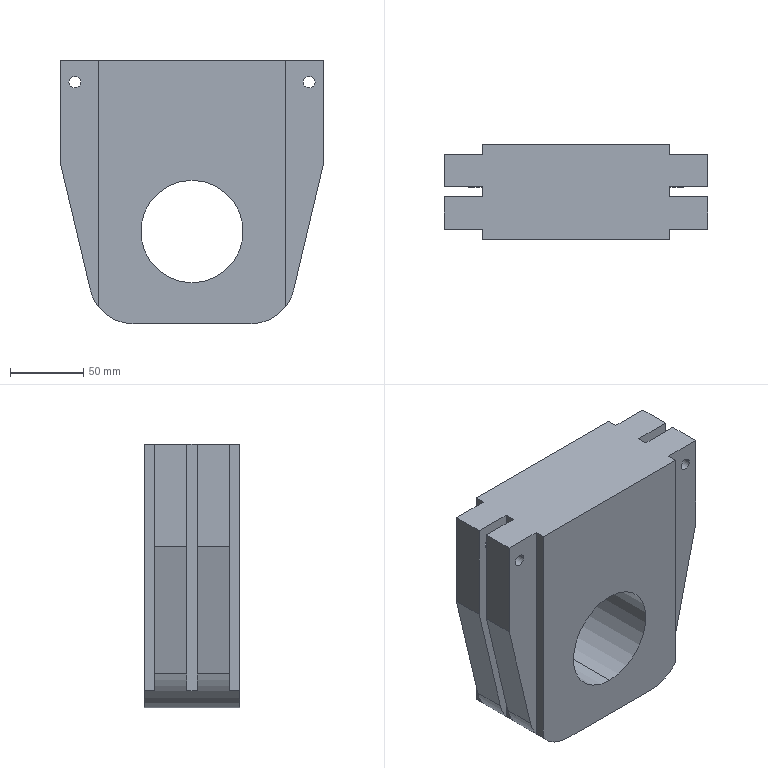Part | SolidWorks | features ICE 4, Extrusion 1 | 1 solid | 38 faces | box 180 x 65 x 180 mm | volume 1515776 mm3 | plane 26 | cylinder 12 | commonest cylinder face diameters 8 x8 60 x2 70 x2
STEP:
#1=CARTESIAN_POINT('',(76.,58.,-15.));
#2=VERTEX_POINT('',#1);
#3=CARTESIAN_POINT('',(84.,58.,-15.));
#4=VERTEX_POINT('',#3);
#5=CARTESIAN_POINT('',(80.,58.,-15.));
#6=DIRECTION('',(0.,-1.,0.));
#7=DIRECTION('',(0.,0.,-1.));
#8=AXIS2_PLACEMENT_3D('',#5,#6,#7);
#9=CIRCLE('',#8,4.);
#10=EDGE_CURVE('',#2,#4,#9,.T.);
#11=ORIENTED_EDGE('',*,*,#10,.F.);
#12=CARTESIAN_POINT('',(76.,36.,-15.));
#13=VERTEX_POINT('',#12);
#14=CARTESIAN_POINT('',(76.,65.,-15.));
#15=DIRECTION('',(0.,-1.,0.));
#16=VECTOR('',#15,1000.);
#17=LINE('',#14,#16);
#18=EDGE_CURVE('',#2,#13,#17,.T.);
#19=ORIENTED_EDGE('',*,*,#18,.T.);
#20=CARTESIAN_POINT('',(84.,36.,-15.));
#21=VERTEX_POINT('',#20);
#22=CARTESIAN_POINT('',(80.,36.,-15.));
#23=DIRECTION('',(0.,-1.,0.));
#24=DIRECTION('',(0.,0.,1.));
#25=AXIS2_PLACEMENT_3D('',#22,#23,#24);
#26=CIRCLE('',#25,4.);
#27=EDGE_CURVE('',#13,#21,#26,.T.);
#28=ORIENTED_EDGE('',*,*,#27,.T.);
#29=CARTESIAN_POINT('',(84.,65.,-15.));
#30=DIRECTION('',(0.,-1.,0.));
#31=VECTOR('',#30,1000.);
#32=LINE('',#29,#31);
#33=EDGE_CURVE('',#4,#21,#32,.T.);
#34=ORIENTED_EDGE('',*,*,#33,.F.);
#35=EDGE_LOOP('',(#11,#19,#28,#34));
#36=FACE_OUTER_BOUND('',#35,.T.);
#37=CARTESIAN_POINT('',(80.,65.,-15.));
#38=DIRECTION('',(0.,-1.,0.));
#39=DIRECTION('',(1.,0.,0.));
#40=AXIS2_PLACEMENT_3D('',#37,#38,#39);
#41=CYLINDRICAL_SURFACE('',#40,4.);
#42=ADVANCED_FACE('',(#36),#41,.F.);
#43=CARTESIAN_POINT('',(-76.,29.,-15.));
#44=VERTEX_POINT('',#43);
#45=CARTESIAN_POINT('',(-84.,29.,-15.));
#46=VERTEX_POINT('',#45);
#47=CARTESIAN_POINT('',(-80.,29.,-15.));
#48=DIRECTION('',(0.,1.,0.));
#49=DIRECTION('',(0.,0.,-1.));
#50=AXIS2_PLACEMENT_3D('',#47,#48,#49);
#51=CIRCLE('',#50,4.);
#52=EDGE_CURVE('',#44,#46,#51,.T.);
#53=ORIENTED_EDGE('',*,*,#52,.T.);
#54=CARTESIAN_POINT('',(-84.,7.,-15.));
#55=VERTEX_POINT('',#54);
#56=CARTESIAN_POINT('',(-84.,65.,-15.));
#57=DIRECTION('',(0.,-1.,0.));
#58=VECTOR('',#57,1000.);
#59=LINE('',#56,#58);
#60=EDGE_CURVE('',#46,#55,#59,.T.);
#61=ORIENTED_EDGE('',*,*,#60,.T.);
#62=CARTESIAN_POINT('',(-76.,7.,-15.));
#63=VERTEX_POINT('',#62);
#64=CARTESIAN_POINT('',(-80.,7.,-15.));
#65=DIRECTION('',(0.,-1.,0.));
#66=DIRECTION('',(1.,0.,0.));
#67=AXIS2_PLACEMENT_3D('',#64,#65,#66);
#68=CIRCLE('',#67,4.);
#69=EDGE_CURVE('',#55,#63,#68,.T.);
#70=ORIENTED_EDGE('',*,*,#69,.T.);
#71=CARTESIAN_POINT('',(-76.,65.,-15.));
#72=DIRECTION('',(0.,-1.,0.));
#73=VECTOR('',#72,1000.);
#74=LINE('',#71,#73);
#75=EDGE_CURVE('',#44,#63,#74,.T.);
#76=ORIENTED_EDGE('',*,*,#75,.F.);
#77=EDGE_LOOP('',(#53,#61,#70,#76));
#78=FACE_OUTER_BOUND('',#77,.T.);
#79=CARTESIAN_POINT('',(-80.,65.,-15.));
#80=DIRECTION('',(0.,-1.,0.));
#81=DIRECTION('',(1.,0.,0.));
#82=AXIS2_PLACEMENT_3D('',#79,#80,#81);
#83=CYLINDRICAL_SURFACE('',#82,4.);
#84=ADVANCED_FACE('',(#78),#83,.F.);
#85=CARTESIAN_POINT('',(0.,0.,-152.));
#86=VERTEX_POINT('',#85);
#87=CARTESIAN_POINT('',(0.,0.,-82.));
#88=VERTEX_POINT('',#87);
#89=CARTESIAN_POINT('',(0.,0.,-117.));
#90=DIRECTION('',(0.,1.,0.));
#91=DIRECTION('',(0.,0.,1.));
#92=AXIS2_PLACEMENT_3D('',#89,#90,#91);
#93=CIRCLE('',#92,35.);
#94=EDGE_CURVE('',#86,#88,#93,.T.);
#95=ORIENTED_EDGE('',*,*,#94,.F.);
#96=CARTESIAN_POINT('',(0.,65.,-152.));
#97=VERTEX_POINT('',#96);
#98=CARTESIAN_POINT('',(0.,0.,-152.));
#99=DIRECTION('',(0.,1.,0.));
#100=VECTOR('',#99,1000.);
#101=LINE('',#98,#100);
#102=EDGE_CURVE('',#86,#97,#101,.T.);
#103=ORIENTED_EDGE('',*,*,#102,.T.);
#104=CARTESIAN_POINT('',(0.,65.,-82.));
#105=VERTEX_POINT('',#104);
#106=CARTESIAN_POINT('',(0.,65.,-117.));
#107=DIRECTION('',(0.,1.,0.));
#108=DIRECTION('',(0.,0.,1.));
#109=AXIS2_PLACEMENT_3D('',#106,#107,#108);
#110=CIRCLE('',#109,35.);
#111=EDGE_CURVE('',#97,#105,#110,.T.);
#112=ORIENTED_EDGE('',*,*,#111,.T.);
#113=CARTESIAN_POINT('',(0.,0.,-82.));
#114=DIRECTION('',(0.,1.,0.));
#115=VECTOR('',#114,1000.);
#116=LINE('',#113,#115);
#117=EDGE_CURVE('',#88,#105,#116,.T.);
#118=ORIENTED_EDGE('',*,*,#117,.F.);
#119=EDGE_LOOP('',(#95,#103,#112,#118));
#120=FACE_OUTER_BOUND('',#119,.T.);
#121=CARTESIAN_POINT('',(0.,0.,-117.));
#122=DIRECTION('',(0.,1.,0.));
#123=DIRECTION('',(0.,0.,1.));
#124=AXIS2_PLACEMENT_3D('',#121,#122,#123);
#125=CYLINDRICAL_SURFACE('',#124,35.);
#126=ADVANCED_FACE('',(#120),#125,.F.);
#127=CARTESIAN_POINT('',(84.,29.,-15.));
#128=VERTEX_POINT('',#127);
#129=CARTESIAN_POINT('',(76.,29.,-15.));
#130=VERTEX_POINT('',#129);
#131=CARTESIAN_POINT('',(80.,29.,-15.));
#132=DIRECTION('',(0.,1.,0.));
#133=DIRECTION('',(1.,0.,0.));
#134=AXIS2_PLACEMENT_3D('',#131,#132,#133);
#135=CIRCLE('',#134,4.);
#136=EDGE_CURVE('',#128,#130,#135,.T.);
#137=ORIENTED_EDGE('',*,*,#136,.T.);
#138=CARTESIAN_POINT('',(76.,7.,-15.));
#139=VERTEX_POINT('',#138);
#140=CARTESIAN_POINT('',(76.,65.,-15.));
#141=DIRECTION('',(0.,-1.,0.));
#142=VECTOR('',#141,1000.);
#143=LINE('',#140,#142);
#144=EDGE_CURVE('',#130,#139,#143,.T.);
#145=ORIENTED_EDGE('',*,*,#144,.T.);
#146=CARTESIAN_POINT('',(84.,7.,-15.));
#147=VERTEX_POINT('',#146);
#148=CARTESIAN_POINT('',(80.,7.,-15.));
#149=DIRECTION('',(0.,-1.,0.));
#150=DIRECTION('',(1.,0.,0.));
#151=AXIS2_PLACEMENT_3D('',#148,#149,#150);
#152=CIRCLE('',#151,4.);
#153=EDGE_CURVE('',#139,#147,#152,.T.);
#154=ORIENTED_EDGE('',*,*,#153,.T.);
#155=CARTESIAN_POINT('',(84.,65.,-15.));
#156=DIRECTION('',(0.,-1.,0.));
#157=VECTOR('',#156,1000.);
#158=LINE('',#155,#157);
#159=EDGE_CURVE('',#128,#147,#158,.T.);
#160=ORIENTED_EDGE('',*,*,#159,.F.);
#161=EDGE_LOOP('',(#137,#145,#154,#160));
#162=FACE_OUTER_BOUND('',#161,.T.);
#163=CARTESIAN_POINT('',(80.,65.,-15.));
#164=DIRECTION('',(0.,-1.,0.));
#165=DIRECTION('',(1.,0.,0.));
#166=AXIS2_PLACEMENT_3D('',#163,#164,#165);
#167=CYLINDRICAL_SURFACE('',#166,4.);
#168=ADVANCED_FACE('',(#162),#167,.F.);
#169=CARTESIAN_POINT('',(-84.,58.,-15.));
#170=VERTEX_POINT('',#169);
#171=CARTESIAN_POINT('',(-76.,58.,-15.));
#172=VERTEX_POINT('',#171);
#173=CARTESIAN_POINT('',(-80.,58.,-15.));
#174=DIRECTION('',(0.,-1.,0.));
#175=DIRECTION('',(0.,0.,-1.));
#176=AXIS2_PLACEMENT_3D('',#173,#174,#175);
#177=CIRCLE('',#176,4.);
#178=EDGE_CURVE('',#170,#172,#177,.T.);
#179=ORIENTED_EDGE('',*,*,#178,.F.);
#180=CARTESIAN_POINT('',(-84.,36.,-15.));
#181=VERTEX_POINT('',#180);
#182=CARTESIAN_POINT('',(-84.,65.,-15.));
#183=DIRECTION('',(0.,-1.,0.));
#184=VECTOR('',#183,1000.);
#185=LINE('',#182,#184);
#186=EDGE_CURVE('',#170,#181,#185,.T.);
#187=ORIENTED_EDGE('',*,*,#186,.T.);
#188=CARTESIAN_POINT('',(-76.,36.,-15.));
#189=VERTEX_POINT('',#188);
#190=CARTESIAN_POINT('',(-80.,36.,-15.));
#191=DIRECTION('',(0.,-1.,0.));
#192=DIRECTION('',(0.,0.,1.));
#193=AXIS2_PLACEMENT_3D('',#190,#191,#192);
#194=CIRCLE('',#193,4.);
#195=EDGE_CURVE('',#181,#189,#194,.T.);
#196=ORIENTED_EDGE('',*,*,#195,.T.);
#197=CARTESIAN_POINT('',(-76.,65.,-15.));
#198=DIRECTION('',(0.,-1.,0.));
#199=VECTOR('',#198,1000.);
#200=LINE('',#197,#199);
#201=EDGE_CURVE('',#172,#189,#200,.T.);
#202=ORIENTED_EDGE('',*,*,#201,.F.);
#203=EDGE_LOOP('',(#179,#187,#196,#202));
#204=FACE_OUTER_BOUND('',#203,.T.);
#205=CARTESIAN_POINT('',(-80.,65.,-15.));
#206=DIRECTION('',(0.,-1.,0.));
#207=DIRECTION('',(1.,0.,0.));
#208=AXIS2_PLACEMENT_3D('',#205,#206,#207);
#209=CYLINDRICAL_SURFACE('',#208,4.);
#210=ADVANCED_FACE('',(#204),#209,.F.);
#211=CARTESIAN_POINT('',(90.,29.,-70.));
#212=VERTEX_POINT('',#211);
#213=CARTESIAN_POINT('',(90.,7.,-70.));
#214=VERTEX_POINT('',#213);
#215=CARTESIAN_POINT('',(90.,65.,-70.));
#216=DIRECTION('',(0.,-1.,0.));
#217=VECTOR('',#216,1000.);
#218=LINE('',#215,#217);
#219=EDGE_CURVE('',#212,#214,#218,.T.);
#220=ORIENTED_EDGE('',*,*,#219,.F.);
#221=CARTESIAN_POINT('',(90.,29.,0.));
#222=VERTEX_POINT('',#221);
#223=CARTESIAN_POINT('',(90.,29.,-180.));
#224=DIRECTION('',(0.,0.,1.));
#225=VECTOR('',#224,1000.);
#226=LINE('',#223,#225);
#227=EDGE_CURVE('',#212,#222,#226,.T.);
#228=ORIENTED_EDGE('',*,*,#227,.T.);
#229=CARTESIAN_POINT('',(90.,7.,0.));
#230=VERTEX_POINT('',#229);
#231=CARTESIAN_POINT('',(90.,65.,0.));
#232=DIRECTION('',(0.,-1.,0.));
#233=VECTOR('',#232,1000.);
#234=LINE('',#231,#233);
#235=EDGE_CURVE('',#222,#230,#234,.T.);
#236=ORIENTED_EDGE('',*,*,#235,.T.);
#237=CARTESIAN_POINT('',(90.,7.,-180.));
#238=DIRECTION('',(0.,0.,1.));
#239=VECTOR('',#238,1000.);
#240=LINE('',#237,#239);
#241=EDGE_CURVE('',#214,#230,#240,.T.);
#242=ORIENTED_EDGE('',*,*,#241,.F.);
#243=EDGE_LOOP('',(#220,#228,#236,#242));
#244=FACE_OUTER_BOUND('',#243,.T.);
#245=CARTESIAN_POINT('',(90.,65.,0.));
#246=DIRECTION('',(-1.,0.,0.));
#247=DIRECTION('',(0.,0.,1.));
#248=AXIS2_PLACEMENT_3D('',#245,#246,#247);
#249=PLANE('',#248);
#250=ADVANCED_FACE('',(#244),#249,.F.);
#251=CARTESIAN_POINT('',(69.444,29.,-156.905));
#252=VERTEX_POINT('',#251);
#253=CARTESIAN_POINT('',(69.444,7.,-156.905));
#254=VERTEX_POINT('',#253);
#255=CARTESIAN_POINT('',(69.444,65.,-156.905));
#256=DIRECTION('',(0.,-1.,0.));
#257=VECTOR('',#256,1000.);
#258=LINE('',#255,#257);
#259=EDGE_CURVE('',#252,#254,#258,.T.);
#260=ORIENTED_EDGE('',*,*,#259,.F.);
#261=CARTESIAN_POINT('',(90.,29.,-70.));
#262=DIRECTION('',(0.2302,0.,0.9731));
#263=VECTOR('',#262,1000.);
#264=LINE('',#261,#263);
#265=EDGE_CURVE('',#252,#212,#264,.T.);
#266=ORIENTED_EDGE('',*,*,#265,.T.);
#267=ORIENTED_EDGE('',*,*,#219,.T.);
#268=CARTESIAN_POINT('',(90.,7.,-70.));
#269=DIRECTION('',(-0.2302,0.,-0.9731));
#270=VECTOR('',#269,1000.);
#271=LINE('',#268,#270);
#272=EDGE_CURVE('',#214,#254,#271,.T.);
#273=ORIENTED_EDGE('',*,*,#272,.T.);
#274=EDGE_LOOP('',(#260,#266,#267,#273));
#275=FACE_OUTER_BOUND('',#274,.T.);
#276=CARTESIAN_POINT('',(90.,65.,-70.));
#277=DIRECTION('',(-0.9731,0.,0.2302));
#278=DIRECTION('',(0.2302,0.,0.9731));
#279=AXIS2_PLACEMENT_3D('',#276,#277,#278);
#280=PLANE('',#279);
#281=ADVANCED_FACE('',(#275),#280,.F.);
#282=CARTESIAN_POINT('',(-69.444,58.,-156.905));
#283=VERTEX_POINT('',#282);
#284=CARTESIAN_POINT('',(-69.444,36.,-156.905));
#285=VERTEX_POINT('',#284);
#286=CARTESIAN_POINT('',(-69.444,65.,-156.905));
#287=DIRECTION('',(0.,-1.,0.));
#288=VECTOR('',#287,1000.);
#289=LINE('',#286,#288);
#290=EDGE_CURVE('',#283,#285,#289,.T.);
#291=ORIENTED_EDGE('',*,*,#290,.T.);
#292=CARTESIAN_POINT('',(-90.,36.,-70.));
#293=VERTEX_POINT('',#292);
#294=CARTESIAN_POINT('',(-90.,36.,-70.));
#295=DIRECTION('',(-0.2302,0.,0.9731));
#296=VECTOR('',#295,1000.);
#297=LINE('',#294,#296);
#298=EDGE_CURVE('',#285,#293,#297,.T.);
#299=ORIENTED_EDGE('',*,*,#298,.T.);
#300=CARTESIAN_POINT('',(-90.,58.,-70.));
#301=VERTEX_POINT('',#300);
#302=CARTESIAN_POINT('',(-90.,65.,-70.));
#303=DIRECTION('',(0.,-1.,0.));
#304=VECTOR('',#303,1000.);
#305=LINE('',#302,#304);
#306=EDGE_CURVE('',#301,#293,#305,.T.);
#307=ORIENTED_EDGE('',*,*,#306,.F.);
#308=CARTESIAN_POINT('',(-90.,58.,-70.));
#309=DIRECTION('',(0.2302,0.,-0.9731));
#310=VECTOR('',#309,1000.);
#311=LINE('',#308,#310);
#312=EDGE_CURVE('',#301,#283,#311,.T.);
#313=ORIENTED_EDGE('',*,*,#312,.T.);
#314=EDGE_LOOP('',(#291,#299,#307,#313));
#315=FACE_OUTER_BOUND('',#314,.T.);
#316=CARTESIAN_POINT('',(-90.,65.,-70.));
#317=DIRECTION('',(0.9731,0.,0.2302));
#318=DIRECTION('',(0.2302,0.,-0.9731));
#319=AXIS2_PLACEMENT_3D('',#316,#317,#318);
#320=PLANE('',#319);
#321=ADVANCED_FACE('',(#315),#320,.F.);
#322=ORIENTED_EDGE('',*,*,#306,.T.);
#323=CARTESIAN_POINT('',(-90.,36.,0.));
#324=VERTEX_POINT('',#323);
#325=CARTESIAN_POINT('',(-90.,36.,-180.));
#326=DIRECTION('',(0.,0.,1.));
#327=VECTOR('',#326,1000.);
#328=LINE('',#325,#327);
#329=EDGE_CURVE('',#293,#324,#328,.T.);
#330=ORIENTED_EDGE('',*,*,#329,.T.);
#331=CARTESIAN_POINT('',(-90.,58.,0.));
#332=VERTEX_POINT('',#331);
#333=CARTESIAN_POINT('',(-90.,65.,0.));
#334=DIRECTION('',(0.,-1.,0.));
#335=VECTOR('',#334,1000.);
#336=LINE('',#333,#335);
#337=EDGE_CURVE('',#332,#324,#336,.T.);
#338=ORIENTED_EDGE('',*,*,#337,.F.);
#339=CARTESIAN_POINT('',(-90.,58.,-180.));
#340=DIRECTION('',(0.,0.,1.));
#341=VECTOR('',#340,1000.);
#342=LINE('',#339,#341);
#343=EDGE_CURVE('',#301,#332,#342,.T.);
#344=ORIENTED_EDGE('',*,*,#343,.F.);
#345=EDGE_LOOP('',(#322,#330,#338,#344));
#346=FACE_OUTER_BOUND('',#345,.T.);
#347=CARTESIAN_POINT('',(-90.,65.,0.));
#348=DIRECTION('',(1.,0.,0.));
#349=DIRECTION('',(0.,0.,-1.));
#350=AXIS2_PLACEMENT_3D('',#347,#348,#349);
#351=PLANE('',#350);
#352=ADVANCED_FACE('',(#346),#351,.F.);
#353=ORIENTED_EDGE('',*,*,#186,.F.);
#354=CARTESIAN_POINT('',(-80.,58.,-15.));
#355=DIRECTION('',(0.,-1.,0.));
#356=DIRECTION('',(0.,0.,-1.));
#357=AXIS2_PLACEMENT_3D('',#354,#355,#356);
#358=CIRCLE('',#357,4.);
#359=EDGE_CURVE('',#172,#170,#358,.T.);
#360=ORIENTED_EDGE('',*,*,#359,.F.);
#361=ORIENTED_EDGE('',*,*,#201,.T.);
#362=CARTESIAN_POINT('',(-80.,36.,-15.));
#363=DIRECTION('',(0.,-1.,0.));
#364=DIRECTION('',(0.,0.,1.));
#365=AXIS2_PLACEMENT_3D('',#362,#363,#364);
#366=CIRCLE('',#365,4.);
#367=EDGE_CURVE('',#189,#181,#366,.T.);
#368=ORIENTED_EDGE('',*,*,#367,.T.);
#369=EDGE_LOOP('',(#353,#360,#361,#368));
#370=FACE_OUTER_BOUND('',#369,.T.);
#371=CARTESIAN_POINT('',(-80.,65.,-15.));
#372=DIRECTION('',(0.,-1.,0.));
#373=DIRECTION('',(1.,0.,0.));
#374=AXIS2_PLACEMENT_3D('',#371,#372,#373);
#375=CYLINDRICAL_SURFACE('',#374,4.);
#376=ADVANCED_FACE('',(#370),#375,.F.);
#377=ORIENTED_EDGE('',*,*,#144,.F.);
#378=CARTESIAN_POINT('',(80.,29.,-15.));
#379=DIRECTION('',(0.,1.,0.));
#380=DIRECTION('',(1.,0.,0.));
#381=AXIS2_PLACEMENT_3D('',#378,#379,#380);
#382=CIRCLE('',#381,4.);
#383=EDGE_CURVE('',#130,#128,#382,.T.);
#384=ORIENTED_EDGE('',*,*,#383,.T.);
#385=ORIENTED_EDGE('',*,*,#159,.T.);
#386=CARTESIAN_POINT('',(80.,7.,-15.));
#387=DIRECTION('',(0.,-1.,0.));
#388=DIRECTION('',(1.,0.,0.));
#389=AXIS2_PLACEMENT_3D('',#386,#387,#388);
#390=CIRCLE('',#389,4.);
#391=EDGE_CURVE('',#147,#139,#390,.T.);
#392=ORIENTED_EDGE('',*,*,#391,.T.);
#393=EDGE_LOOP('',(#377,#384,#385,#392));
#394=FACE_OUTER_BOUND('',#393,.T.);
#395=CARTESIAN_POINT('',(80.,65.,-15.));
#396=DIRECTION('',(0.,-1.,0.));
#397=DIRECTION('',(1.,0.,0.));
#398=AXIS2_PLACEMENT_3D('',#395,#396,#397);
#399=CYLINDRICAL_SURFACE('',#398,4.);
#400=ADVANCED_FACE('',(#394),#399,.F.);
#401=CARTESIAN_POINT('',(90.,58.,0.));
#402=VERTEX_POINT('',#401);
#403=CARTESIAN_POINT('',(90.,36.,0.));
#404=VERTEX_POINT('',#403);
#405=CARTESIAN_POINT('',(90.,65.,0.));
#406=DIRECTION('',(0.,-1.,0.));
#407=VECTOR('',#406,1000.);
#408=LINE('',#405,#407);
#409=EDGE_CURVE('',#402,#404,#408,.T.);
#410=ORIENTED_EDGE('',*,*,#409,.T.);
#411=CARTESIAN_POINT('',(90.,36.,-70.));
#412=VERTEX_POINT('',#411);
#413=CARTESIAN_POINT('',(90.,36.,-180.));
#414=DIRECTION('',(0.,0.,1.));
#415=VECTOR('',#414,1000.);
#416=LINE('',#413,#415);
#417=EDGE_CURVE('',#412,#404,#416,.T.);
#418=ORIENTED_EDGE('',*,*,#417,.F.);
#419=CARTESIAN_POINT('',(90.,58.,-70.));
#420=VERTEX_POINT('',#419);
#421=CARTESIAN_POINT('',(90.,65.,-70.));
#422=DIRECTION('',(0.,-1.,0.));
#423=VECTOR('',#422,1000.);
#424=LINE('',#421,#423);
#425=EDGE_CURVE('',#420,#412,#424,.T.);
#426=ORIENTED_EDGE('',*,*,#425,.F.);
#427=CARTESIAN_POINT('',(90.,58.,-180.));
#428=DIRECTION('',(0.,0.,1.));
#429=VECTOR('',#428,1000.);
#430=LINE('',#427,#429);
#431=EDGE_CURVE('',#420,#402,#430,.T.);
#432=ORIENTED_EDGE('',*,*,#431,.T.);
#433=EDGE_LOOP('',(#410,#418,#426,#432));
#434=FACE_OUTER_BOUND('',#433,.T.);
#435=CARTESIAN_POINT('',(90.,65.,0.));
#436=DIRECTION('',(-1.,0.,0.));
#437=DIRECTION('',(0.,0.,1.));
#438=AXIS2_PLACEMENT_3D('',#435,#436,#437);
#439=PLANE('',#438);
#440=ADVANCED_FACE('',(#434),#439,.F.);
#441=ORIENTED_EDGE('',*,*,#425,.T.);
#442=CARTESIAN_POINT('',(69.444,36.,-156.905));
#443=VERTEX_POINT('',#442);
#444=CARTESIAN_POINT('',(90.,36.,-70.));
#445=DIRECTION('',(-0.2302,0.,-0.9731));
#446=VECTOR('',#445,1000.);
#447=LINE('',#444,#446);
#448=EDGE_CURVE('',#412,#443,#447,.T.);
#449=ORIENTED_EDGE('',*,*,#448,.T.);
#450=CARTESIAN_POINT('',(69.444,58.,-156.905));
#451=VERTEX_POINT('',#450);
#452=CARTESIAN_POINT('',(69.444,65.,-156.905));
#453=DIRECTION('',(0.,-1.,0.));
#454=VECTOR('',#453,1000.);
#455=LINE('',#452,#454);
#456=EDGE_CURVE('',#451,#443,#455,.T.);
#457=ORIENTED_EDGE('',*,*,#456,.F.);
#458=CARTESIAN_POINT('',(90.,58.,-70.));
#459=DIRECTION('',(0.2302,0.,0.9731));
#460=VECTOR('',#459,1000.);
#461=LINE('',#458,#460);
#462=EDGE_CURVE('',#451,#420,#461,.T.);
#463=ORIENTED_EDGE('',*,*,#462,.T.);
#464=EDGE_LOOP('',(#441,#449,#457,#463));
#465=FACE_OUTER_BOUND('',#464,.T.);
#466=CARTESIAN_POINT('',(90.,65.,-70.));
#467=DIRECTION('',(-0.9731,0.,0.2302));
#468=DIRECTION('',(0.2302,0.,0.9731));
#469=AXIS2_PLACEMENT_3D('',#466,#467,#468);
#470=PLANE('',#469);
#471=ADVANCED_FACE('',(#465),#470,.F.);
#472=CARTESIAN_POINT('',(64.,36.,-168.329));
#473=VERTEX_POINT('',#472);
#474=CARTESIAN_POINT('',(64.,29.,-168.329));
#475=VERTEX_POINT('',#474);
#476=CARTESIAN_POINT('',(64.,65.,-168.329));
#477=DIRECTION('',(0.,-1.,0.));
#478=VECTOR('',#477,1000.);
#479=LINE('',#476,#478);
#480=EDGE_CURVE('',#473,#475,#479,.T.);
#481=ORIENTED_EDGE('',*,*,#480,.T.);
#482=CARTESIAN_POINT('',(40.25,29.,-150.));
#483=DIRECTION('',(0.,-1.,0.));
#484=DIRECTION('',(1.,0.,0.));
#485=AXIS2_PLACEMENT_3D('',#482,#483,#484);
#486=CIRCLE('',#485,30.);
#487=EDGE_CURVE('',#475,#252,#486,.T.);
#488=ORIENTED_EDGE('',*,*,#487,.T.);
#489=ORIENTED_EDGE('',*,*,#259,.T.);
#490=CARTESIAN_POINT('',(64.,7.,-168.329));
#491=VERTEX_POINT('',#490);
#492=CARTESIAN_POINT('',(40.25,7.,-150.));
#493=DIRECTION('',(0.,1.,0.));
#494=DIRECTION('',(-1.,0.,0.));
#495=AXIS2_PLACEMENT_3D('',#492,#493,#494);
#496=CIRCLE('',#495,30.);
#497=EDGE_CURVE('',#254,#491,#496,.T.);
#498=ORIENTED_EDGE('',*,*,#497,.T.);
#499=CARTESIAN_POINT('',(64.,0.,-168.329));
#500=VERTEX_POINT('',#499);
#501=CARTESIAN_POINT('',(64.,65.,-168.329));
#502=DIRECTION('',(0.,-1.,0.));
#503=VECTOR('',#502,1000.);
#504=LINE('',#501,#503);
#505=EDGE_CURVE('',#491,#500,#504,.T.);
#506=ORIENTED_EDGE('',*,*,#505,.T.);
#507=CARTESIAN_POINT('',(40.25,0.,-180.));
#508=VERTEX_POINT('',#507);
#509=CARTESIAN_POINT('',(40.25,0.,-150.));
#510=DIRECTION('',(0.,1.,0.));
#511=DIRECTION('',(0.,0.,-1.));
#512=AXIS2_PLACEMENT_3D('',#509,#510,#511);
#513=CIRCLE('',#512,30.);
#514=EDGE_CURVE('',#500,#508,#513,.T.);
#515=ORIENTED_EDGE('',*,*,#514,.T.);
#516=CARTESIAN_POINT('',(40.25,65.,-180.));
#517=VERTEX_POINT('',#516);
#518=CARTESIAN_POINT('',(40.25,65.,-180.));
#519=DIRECTION('',(0.,-1.,0.));
#520=VECTOR('',#519,1000.);
#521=LINE('',#518,#520);
#522=EDGE_CURVE('',#517,#508,#521,.T.);
#523=ORIENTED_EDGE('',*,*,#522,.F.);
#524=CARTESIAN_POINT('',(64.,65.,-168.329));
#525=VERTEX_POINT('',#524);
#526=CARTESIAN_POINT('',(40.25,65.,-150.));
#527=DIRECTION('',(0.,1.,0.));
#528=DIRECTION('',(0.,0.,-1.));
#529=AXIS2_PLACEMENT_3D('',#526,#527,#528);
#530=CIRCLE('',#529,30.);
#531=EDGE_CURVE('',#525,#517,#530,.T.);
#532=ORIENTED_EDGE('',*,*,#531,.F.);
#533=CARTESIAN_POINT('',(64.,58.,-168.329));
#534=VERTEX_POINT('',#533);
#535=CARTESIAN_POINT('',(64.,65.,-168.329));
#536=DIRECTION('',(0.,-1.,0.));
#537=VECTOR('',#536,1000.);
#538=LINE('',#535,#537);
#539=EDGE_CURVE('',#525,#534,#538,.T.);
#540=ORIENTED_EDGE('',*,*,#539,.T.);
#541=CARTESIAN_POINT('',(40.25,58.,-150.));
#542=DIRECTION('',(0.,-1.,0.));
#543=DIRECTION('',(0.,0.,-1.));
#544=AXIS2_PLACEMENT_3D('',#541,#542,#543);
#545=CIRCLE('',#544,30.);
#546=EDGE_CURVE('',#534,#451,#545,.T.);
#547=ORIENTED_EDGE('',*,*,#546,.T.);
#548=ORIENTED_EDGE('',*,*,#456,.T.);
#549=CARTESIAN_POINT('',(40.25,36.,-150.));
#550=DIRECTION('',(0.,1.,0.));
#551=DIRECTION('',(0.,0.,1.));
#552=AXIS2_PLACEMENT_3D('',#549,#550,#551);
#553=CIRCLE('',#552,30.);
#554=EDGE_CURVE('',#443,#473,#553,.T.);
#555=ORIENTED_EDGE('',*,*,#554,.T.);
#556=EDGE_LOOP('',(#481,#488,#489,#498,#506,#515,#523,#532,#540,#547,#548,#555));
#557=FACE_OUTER_BOUND('',#556,.T.);
#558=CARTESIAN_POINT('',(40.25,65.,-150.));
#559=DIRECTION('',(0.,-1.,0.));
#560=DIRECTION('',(0.,0.,-1.));
#561=AXIS2_PLACEMENT_3D('',#558,#559,#560);
#562=CYLINDRICAL_SURFACE('',#561,30.);
#563=ADVANCED_FACE('',(#557),#562,.T.);
#564=CARTESIAN_POINT('',(-40.25,0.,-180.));
#565=VERTEX_POINT('',#564);
#566=CARTESIAN_POINT('',(-40.25,0.,-180.));
#567=DIRECTION('',(-1.,0.,0.));
#568=VECTOR('',#567,1000.);
#569=LINE('',#566,#568);
#570=EDGE_CURVE('',#508,#565,#569,.T.);
#571=ORIENTED_EDGE('',*,*,#570,.T.);
#572=CARTESIAN_POINT('',(-40.25,65.,-180.));
#573=VERTEX_POINT('',#572);
#574=CARTESIAN_POINT('',(-40.25,65.,-180.));
#575=DIRECTION('',(0.,-1.,0.));
#576=VECTOR('',#575,1000.);
#577=LINE('',#574,#576);
#578=EDGE_CURVE('',#573,#565,#577,.T.);
#579=ORIENTED_EDGE('',*,*,#578,.F.);
#580=CARTESIAN_POINT('',(-40.25,65.,-180.));
#581=DIRECTION('',(-1.,0.,0.));
#582=VECTOR('',#581,1000.);
#583=LINE('',#580,#582);
#584=EDGE_CURVE('',#517,#573,#583,.T.);
#585=ORIENTED_EDGE('',*,*,#584,.F.);
#586=ORIENTED_EDGE('',*,*,#522,.T.);
#587=EDGE_LOOP('',(#571,#579,#585,#586));
#588=FACE_OUTER_BOUND('',#587,.T.);
#589=CARTESIAN_POINT('',(-40.25,65.,-180.));
#590=DIRECTION('',(0.,0.,1.));
#591=DIRECTION('',(1.,0.,0.));
#592=AXIS2_PLACEMENT_3D('',#589,#590,#591);
#593=PLANE('',#592);
#594=ADVANCED_FACE('',(#588),#593,.F.);
#595=CARTESIAN_POINT('',(-64.,29.,-168.329));
#596=VERTEX_POINT('',#595);
#597=CARTESIAN_POINT('',(-64.,36.,-168.329));
#598=VERTEX_POINT('',#597);
#599=CARTESIAN_POINT('',(-64.,65.,-168.329));
#600=DIRECTION('',(0.,1.,0.));
#601=VECTOR('',#600,1000.);
#602=LINE('',#599,#601);
#603=EDGE_CURVE('',#596,#598,#602,.T.);
#604=ORIENTED_EDGE('',*,*,#603,.T.);
#605=CARTESIAN_POINT('',(-40.25,36.,-150.));
#606=DIRECTION('',(0.,1.,0.));
#607=DIRECTION('',(0.,0.,1.));
#608=AXIS2_PLACEMENT_3D('',#605,#606,#607);
#609=CIRCLE('',#608,30.);
#610=EDGE_CURVE('',#598,#285,#609,.T.);
#611=ORIENTED_EDGE('',*,*,#610,.T.);
#612=ORIENTED_EDGE('',*,*,#290,.F.);
#613=CARTESIAN_POINT('',(-64.,58.,-168.329));
#614=VERTEX_POINT('',#613);
#615=CARTESIAN_POINT('',(-40.25,58.,-150.));
#616=DIRECTION('',(0.,-1.,0.));
#617=DIRECTION('',(0.,0.,-1.));
#618=AXIS2_PLACEMENT_3D('',#615,#616,#617);
#619=CIRCLE('',#618,30.);
#620=EDGE_CURVE('',#283,#614,#619,.T.);
#621=ORIENTED_EDGE('',*,*,#620,.T.);
#622=CARTESIAN_POINT('',(-64.,65.,-168.329));
#623=VERTEX_POINT('',#622);
#624=CARTESIAN_POINT('',(-64.,65.,-168.329));
#625=DIRECTION('',(0.,1.,0.));
#626=VECTOR('',#625,1000.);
#627=LINE('',#624,#626);
#628=EDGE_CURVE('',#614,#623,#627,.T.);
#629=ORIENTED_EDGE('',*,*,#628,.T.);
#630=CARTESIAN_POINT('',(-40.25,65.,-150.));
#631=DIRECTION('',(0.,1.,0.));
#632=DIRECTION('',(0.,0.,1.));
#633=AXIS2_PLACEMENT_3D('',#630,#631,#632);
#634=CIRCLE('',#633,30.);
#635=EDGE_CURVE('',#573,#623,#634,.T.);
#636=ORIENTED_EDGE('',*,*,#635,.F.);
#637=ORIENTED_EDGE('',*,*,#578,.T.);
#638=CARTESIAN_POINT('',(-64.,0.,-168.329));
#639=VERTEX_POINT('',#638);
#640=CARTESIAN_POINT('',(-40.25,0.,-150.));
#641=DIRECTION('',(0.,1.,0.));
#642=DIRECTION('',(0.,0.,1.));
#643=AXIS2_PLACEMENT_3D('',#640,#641,#642);
#644=CIRCLE('',#643,30.);
#645=EDGE_CURVE('',#565,#639,#644,.T.);
#646=ORIENTED_EDGE('',*,*,#645,.T.);
#647=CARTESIAN_POINT('',(-64.,7.,-168.329));
#648=VERTEX_POINT('',#647);
#649=CARTESIAN_POINT('',(-64.,65.,-168.329));
#650=DIRECTION('',(0.,1.,0.));
#651=VECTOR('',#650,1000.);
#652=LINE('',#649,#651);
#653=EDGE_CURVE('',#639,#648,#652,.T.);
#654=ORIENTED_EDGE('',*,*,#653,.T.);
#655=CARTESIAN_POINT('',(-69.444,7.,-156.905));
#656=VERTEX_POINT('',#655);
#657=CARTESIAN_POINT('',(-40.25,7.,-150.));
#658=DIRECTION('',(0.,1.,0.));
#659=DIRECTION('',(0.,0.,1.));
#660=AXIS2_PLACEMENT_3D('',#657,#658,#659);
#661=CIRCLE('',#660,30.);
#662=EDGE_CURVE('',#648,#656,#661,.T.);
#663=ORIENTED_EDGE('',*,*,#662,.T.);
#664=CARTESIAN_POINT('',(-69.444,29.,-156.905));
#665=VERTEX_POINT('',#664);
#666=CARTESIAN_POINT('',(-69.444,65.,-156.905));
#667=DIRECTION('',(0.,-1.,0.));
#668=VECTOR('',#667,1000.);
#669=LINE('',#666,#668);
#670=EDGE_CURVE('',#665,#656,#669,.T.);
#671=ORIENTED_EDGE('',*,*,#670,.F.);
#672=CARTESIAN_POINT('',(-40.25,29.,-150.));
#673=DIRECTION('',(0.,-1.,0.));
#674=DIRECTION('',(0.,0.,-1.));
#675=AXIS2_PLACEMENT_3D('',#672,#673,#674);
#676=CIRCLE('',#675,30.);
#677=EDGE_CURVE('',#665,#596,#676,.T.);
#678=ORIENTED_EDGE('',*,*,#677,.T.);
#679=EDGE_LOOP('',(#604,#611,#612,#621,#629,#636,#637,#646,#654,#663,#671,#678));
#680=FACE_OUTER_BOUND('',#679,.T.);
#681=CARTESIAN_POINT('',(-40.25,65.,-150.));
#682=DIRECTION('',(0.,-1.,0.));
#683=DIRECTION('',(0.,0.,-1.));
#684=AXIS2_PLACEMENT_3D('',#681,#682,#683);
#685=CYLINDRICAL_SURFACE('',#684,30.);
#686=ADVANCED_FACE('',(#680),#685,.T.);
#687=CARTESIAN_POINT('',(-90.,29.,-70.));
#688=VERTEX_POINT('',#687);
#689=CARTESIAN_POINT('',(-90.,7.,-70.));
#690=VERTEX_POINT('',#689);
#691=CARTESIAN_POINT('',(-90.,65.,-70.));
#692=DIRECTION('',(0.,-1.,0.));
#693=VECTOR('',#692,1000.);
#694=LINE('',#691,#693);
#695=EDGE_CURVE('',#688,#690,#694,.T.);
#696=ORIENTED_EDGE('',*,*,#695,.F.);
#697=CARTESIAN_POINT('',(-90.,29.,-70.));
#698=DIRECTION('',(0.2302,0.,-0.9731));
#699=VECTOR('',#698,1000.);
#700=LINE('',#697,#699);
#701=EDGE_CURVE('',#688,#665,#700,.T.);
#702=ORIENTED_EDGE('',*,*,#701,.T.);
#703=ORIENTED_EDGE('',*,*,#670,.T.);
#704=CARTESIAN_POINT('',(-90.,7.,-70.));
#705=DIRECTION('',(-0.2302,0.,0.9731));
#706=VECTOR('',#705,1000.);
#707=LINE('',#704,#706);
#708=EDGE_CURVE('',#656,#690,#707,.T.);
#709=ORIENTED_EDGE('',*,*,#708,.T.);
#710=EDGE_LOOP('',(#696,#702,#703,#709));
#711=FACE_OUTER_BOUND('',#710,.T.);
#712=CARTESIAN_POINT('',(-90.,65.,-70.));
#713=DIRECTION('',(0.9731,0.,0.2302));
#714=DIRECTION('',(0.2302,0.,-0.9731));
#715=AXIS2_PLACEMENT_3D('',#712,#713,#714);
#716=PLANE('',#715);
#717=ADVANCED_FACE('',(#711),#716,.F.);
#718=CARTESIAN_POINT('',(-90.,29.,0.));
#719=VERTEX_POINT('',#718);
#720=CARTESIAN_POINT('',(-90.,7.,0.));
#721=VERTEX_POINT('',#720);
#722=CARTESIAN_POINT('',(-90.,65.,0.));
#723=DIRECTION('',(0.,-1.,0.));
#724=VECTOR('',#723,1000.);
#725=LINE('',#722,#724);
#726=EDGE_CURVE('',#719,#721,#725,.T.);
#727=ORIENTED_EDGE('',*,*,#726,.F.);
#728=CARTESIAN_POINT('',(-90.,29.,-180.));
#729=DIRECTION('',(0.,0.,1.));
#730=VECTOR('',#729,1000.);
#731=LINE('',#728,#730);
#732=EDGE_CURVE('',#688,#719,#731,.T.);
#733=ORIENTED_EDGE('',*,*,#732,.F.);
#734=ORIENTED_EDGE('',*,*,#695,.T.);
#735=CARTESIAN_POINT('',(-90.,7.,-180.));
#736=DIRECTION('',(0.,0.,1.));
#737=VECTOR('',#736,1000.);
#738=LINE('',#735,#737);
#739=EDGE_CURVE('',#690,#721,#738,.T.);
#740=ORIENTED_EDGE('',*,*,#739,.T.);
#741=EDGE_LOOP('',(#727,#733,#734,#740));
#742=FACE_OUTER_BOUND('',#741,.T.);
#743=CARTESIAN_POINT('',(-90.,65.,0.));
#744=DIRECTION('',(1.,0.,0.));
#745=DIRECTION('',(0.,0.,-1.));
#746=AXIS2_PLACEMENT_3D('',#743,#744,#745);
#747=PLANE('',#746);
#748=ADVANCED_FACE('',(#742),#747,.F.);
#749=ORIENTED_EDGE('',*,*,#337,.T.);
#750=CARTESIAN_POINT('',(-64.,36.,0.));
#751=VERTEX_POINT('',#750);
#752=CARTESIAN_POINT('',(-90.,36.,0.));
#753=DIRECTION('',(-1.,0.,0.));
#754=VECTOR('',#753,1000.);
#755=LINE('',#752,#754);
#756=EDGE_CURVE('',#751,#324,#755,.T.);
#757=ORIENTED_EDGE('',*,*,#756,.F.);
#758=CARTESIAN_POINT('',(-64.,29.,0.));
#759=VERTEX_POINT('',#758);
#760=CARTESIAN_POINT('',(-64.,36.,0.));
#761=DIRECTION('',(0.,1.,0.));
#762=VECTOR('',#761,1000.);
#763=LINE('',#760,#762);
#764=EDGE_CURVE('',#759,#751,#763,.T.);
#765=ORIENTED_EDGE('',*,*,#764,.F.);
#766=CARTESIAN_POINT('',(-90.,29.,0.));
#767=DIRECTION('',(1.,0.,0.));
#768=VECTOR('',#767,1000.);
#769=LINE('',#766,#768);
#770=EDGE_CURVE('',#719,#759,#769,.T.);
#771=ORIENTED_EDGE('',*,*,#770,.F.);
#772=ORIENTED_EDGE('',*,*,#726,.T.);
#773=CARTESIAN_POINT('',(-64.,7.,0.));
#774=VERTEX_POINT('',#773);
#775=CARTESIAN_POINT('',(-90.,7.,0.));
#776=DIRECTION('',(-1.,0.,0.));
#777=VECTOR('',#776,1000.);
#778=LINE('',#775,#777);
#779=EDGE_CURVE('',#774,#721,#778,.T.);
#780=ORIENTED_EDGE('',*,*,#779,.F.);
#781=CARTESIAN_POINT('',(-64.,0.,0.));
#782=VERTEX_POINT('',#781);
#783=CARTESIAN_POINT('',(-64.,0.,0.));
#784=DIRECTION('',(0.,1.,0.));
#785=VECTOR('',#784,1000.);
#786=LINE('',#783,#785);
#787=EDGE_CURVE('',#782,#774,#786,.T.);
#788=ORIENTED_EDGE('',*,*,#787,.F.);
#789=CARTESIAN_POINT('',(64.,0.,0.));
#790=VERTEX_POINT('',#789);
#791=CARTESIAN_POINT('',(-90.,0.,0.));
#792=DIRECTION('',(1.,0.,0.));
#793=VECTOR('',#792,1000.);
#794=LINE('',#791,#793);
#795=EDGE_CURVE('',#782,#790,#794,.T.);
#796=ORIENTED_EDGE('',*,*,#795,.T.);
#797=CARTESIAN_POINT('',(64.,7.,0.));
#798=VERTEX_POINT('',#797);
#799=CARTESIAN_POINT('',(64.,0.,0.));
#800=DIRECTION('',(0.,-1.,0.));
#801=VECTOR('',#800,1000.);
#802=LINE('',#799,#801);
#803=EDGE_CURVE('',#798,#790,#802,.T.);
#804=ORIENTED_EDGE('',*,*,#803,.F.);
#805=CARTESIAN_POINT('',(90.,7.,0.));
#806=DIRECTION('',(-1.,0.,0.));
#807=VECTOR('',#806,1000.);
#808=LINE('',#805,#807);
#809=EDGE_CURVE('',#230,#798,#808,.T.);
#810=ORIENTED_EDGE('',*,*,#809,.F.);
#811=ORIENTED_EDGE('',*,*,#235,.F.);
#812=CARTESIAN_POINT('',(64.,29.,0.));
#813=VERTEX_POINT('',#812);
#814=CARTESIAN_POINT('',(90.,29.,0.));
#815=DIRECTION('',(1.,0.,0.));
#816=VECTOR('',#815,1000.);
#817=LINE('',#814,#816);
#818=EDGE_CURVE('',#813,#222,#817,.T.);
#819=ORIENTED_EDGE('',*,*,#818,.F.);
#820=CARTESIAN_POINT('',(64.,36.,0.));
#821=VERTEX_POINT('',#820);
#822=CARTESIAN_POINT('',(64.,36.,0.));
#823=DIRECTION('',(0.,-1.,0.));
#824=VECTOR('',#823,1000.);
#825=LINE('',#822,#824);
#826=EDGE_CURVE('',#821,#813,#825,.T.);
#827=ORIENTED_EDGE('',*,*,#826,.F.);
#828=CARTESIAN_POINT('',(90.,36.,0.));
#829=DIRECTION('',(-1.,0.,0.));
#830=VECTOR('',#829,1000.);
#831=LINE('',#828,#830);
#832=EDGE_CURVE('',#404,#821,#831,.T.);
#833=ORIENTED_EDGE('',*,*,#832,.F.);
#834=ORIENTED_EDGE('',*,*,#409,.F.);
#835=CARTESIAN_POINT('',(64.,58.,0.));
#836=VERTEX_POINT('',#835);
#837=CARTESIAN_POINT('',(90.,58.,0.));
#838=DIRECTION('',(1.,0.,0.));
#839=VECTOR('',#838,1000.);
#840=LINE('',#837,#839);
#841=EDGE_CURVE('',#836,#402,#840,.T.);
#842=ORIENTED_EDGE('',*,*,#841,.F.);
#843=CARTESIAN_POINT('',(64.,65.,0.));
#844=VERTEX_POINT('',#843);
#845=CARTESIAN_POINT('',(64.,65.,0.));
#846=DIRECTION('',(0.,-1.,0.));
#847=VECTOR('',#846,1000.);
#848=LINE('',#845,#847);
#849=EDGE_CURVE('',#844,#836,#848,.T.);
#850=ORIENTED_EDGE('',*,*,#849,.F.);
#851=CARTESIAN_POINT('',(-64.,65.,0.));
#852=VERTEX_POINT('',#851);
#853=CARTESIAN_POINT('',(-90.,65.,0.));
#854=DIRECTION('',(1.,0.,0.));
#855=VECTOR('',#854,1000.);
#856=LINE('',#853,#855);
#857=EDGE_CURVE('',#852,#844,#856,.T.);
#858=ORIENTED_EDGE('',*,*,#857,.F.);
#859=CARTESIAN_POINT('',(-64.,58.,0.));
#860=VERTEX_POINT('',#859);
#861=CARTESIAN_POINT('',(-64.,65.,0.));
#862=DIRECTION('',(0.,1.,0.));
#863=VECTOR('',#862,1000.);
#864=LINE('',#861,#863);
#865=EDGE_CURVE('',#860,#852,#864,.T.);
#866=ORIENTED_EDGE('',*,*,#865,.F.);
#867=CARTESIAN_POINT('',(-90.,58.,0.));
#868=DIRECTION('',(1.,0.,0.));
#869=VECTOR('',#868,1000.);
#870=LINE('',#867,#869);
#871=EDGE_CURVE('',#332,#860,#870,.T.);
#872=ORIENTED_EDGE('',*,*,#871,.F.);
#873=EDGE_LOOP('',(#749,#757,#765,#771,#772,#780,#788,#796,#804,#810,#811,#819,#827,#833,#834,#842,#850,#858,#866,#872));
#874=FACE_OUTER_BOUND('',#873,.T.);
#875=CARTESIAN_POINT('',(-90.,65.,0.));
#876=DIRECTION('',(0.,0.,-1.));
#877=DIRECTION('',(-1.,0.,0.));
#878=AXIS2_PLACEMENT_3D('',#875,#876,#877);
#879=PLANE('',#878);
#880=ADVANCED_FACE('',(#874),#879,.F.);
#881=CARTESIAN_POINT('',(0.,65.,-117.));
#882=DIRECTION('',(0.,1.,0.));
#883=DIRECTION('',(0.,0.,1.));
#884=AXIS2_PLACEMENT_3D('',#881,#882,#883);
#885=CIRCLE('',#884,35.);
#886=EDGE_CURVE('',#105,#97,#885,.T.);
#887=ORIENTED_EDGE('',*,*,#886,.F.);
#888=ORIENTED_EDGE('',*,*,#111,.F.);
#889=EDGE_LOOP('',(#887,#888));
#890=FACE_BOUND('',#889,.T.);
#891=ORIENTED_EDGE('',*,*,#635,.T.);
#892=CARTESIAN_POINT('',(-64.,65.,-150.));
#893=DIRECTION('',(0.,0.,1.));
#894=VECTOR('',#893,1000.);
#895=LINE('',#892,#894);
#896=EDGE_CURVE('',#623,#852,#895,.T.);
#897=ORIENTED_EDGE('',*,*,#896,.T.);
#898=ORIENTED_EDGE('',*,*,#857,.T.);
#899=CARTESIAN_POINT('',(64.,65.,-150.));
#900=DIRECTION('',(0.,0.,-1.));
#901=VECTOR('',#900,1000.);
#902=LINE('',#899,#901);
#903=EDGE_CURVE('',#844,#525,#902,.T.);
#904=ORIENTED_EDGE('',*,*,#903,.T.);
#905=ORIENTED_EDGE('',*,*,#531,.T.);
#906=ORIENTED_EDGE('',*,*,#584,.T.);
#907=EDGE_LOOP('',(#891,#897,#898,#904,#905,#906));
#908=FACE_OUTER_BOUND('',#907,.T.);
#909=CARTESIAN_POINT('',(40.25,65.,-150.));
#910=DIRECTION('',(0.,-1.,0.));
#911=DIRECTION('',(0.,0.,-1.));
#912=AXIS2_PLACEMENT_3D('',#909,#910,#911);
#913=PLANE('',#912);
#914=ADVANCED_FACE('',(#890,#908),#913,.F.);
#915=CARTESIAN_POINT('',(-64.,0.,-150.));
#916=DIRECTION('',(0.,0.,1.));
#917=VECTOR('',#916,1000.);
#918=LINE('',#915,#917);
#919=EDGE_CURVE('',#639,#782,#918,.T.);
#920=ORIENTED_EDGE('',*,*,#919,.F.);
#921=ORIENTED_EDGE('',*,*,#645,.F.);
#922=ORIENTED_EDGE('',*,*,#570,.F.);
#923=ORIENTED_EDGE('',*,*,#514,.F.);
#924=CARTESIAN_POINT('',(64.,0.,-150.));
#925=DIRECTION('',(0.,0.,-1.));
#926=VECTOR('',#925,1000.);
#927=LINE('',#924,#926);
#928=EDGE_CURVE('',#790,#500,#927,.T.);
#929=ORIENTED_EDGE('',*,*,#928,.F.);
#930=ORIENTED_EDGE('',*,*,#795,.F.);
#931=EDGE_LOOP('',(#920,#921,#922,#923,#929,#930));
#932=FACE_OUTER_BOUND('',#931,.T.);
#933=CARTESIAN_POINT('',(0.,0.,-117.));
#934=DIRECTION('',(0.,1.,0.));
#935=DIRECTION('',(0.,0.,1.));
#936=AXIS2_PLACEMENT_3D('',#933,#934,#935);
#937=CIRCLE('',#936,35.);
#938=EDGE_CURVE('',#88,#86,#937,.T.);
#939=ORIENTED_EDGE('',*,*,#938,.T.);
#940=ORIENTED_EDGE('',*,*,#94,.T.);
#941=EDGE_LOOP('',(#939,#940));
#942=FACE_BOUND('',#941,.T.);
#943=CARTESIAN_POINT('',(40.25,0.,-150.));
#944=DIRECTION('',(0.,-1.,0.));
#945=DIRECTION('',(0.,0.,-1.));
#946=AXIS2_PLACEMENT_3D('',#943,#944,#945);
#947=PLANE('',#946);
#948=ADVANCED_FACE('',(#932,#942),#947,.T.);
#949=ORIENTED_EDGE('',*,*,#102,.F.);
#950=ORIENTED_EDGE('',*,*,#938,.F.);
#951=ORIENTED_EDGE('',*,*,#117,.T.);
#952=ORIENTED_EDGE('',*,*,#886,.T.);
#953=EDGE_LOOP('',(#949,#950,#951,#952));
#954=FACE_OUTER_BOUND('',#953,.T.);
#955=CARTESIAN_POINT('',(0.,0.,-117.));
#956=DIRECTION('',(0.,1.,0.));
#957=DIRECTION('',(0.,0.,1.));
#958=AXIS2_PLACEMENT_3D('',#955,#956,#957);
#959=CYLINDRICAL_SURFACE('',#958,35.);
#960=ADVANCED_FACE('',(#954),#959,.F.);
#961=ORIENTED_EDGE('',*,*,#391,.F.);
#962=ORIENTED_EDGE('',*,*,#153,.F.);
#963=EDGE_LOOP('',(#961,#962));
#964=FACE_BOUND('',#963,.T.);
#965=ORIENTED_EDGE('',*,*,#241,.T.);
#966=ORIENTED_EDGE('',*,*,#809,.T.);
#967=CARTESIAN_POINT('',(64.,7.,-180.));
#968=DIRECTION('',(0.,0.,1.));
#969=VECTOR('',#968,1000.);
#970=LINE('',#967,#969);
#971=EDGE_CURVE('',#491,#798,#970,.T.);
#972=ORIENTED_EDGE('',*,*,#971,.F.);
#973=ORIENTED_EDGE('',*,*,#497,.F.);
#974=ORIENTED_EDGE('',*,*,#272,.F.);
#975=EDGE_LOOP('',(#965,#966,#972,#973,#974));
#976=FACE_OUTER_BOUND('',#975,.T.);
#977=CARTESIAN_POINT('',(90.,7.,-180.));
#978=DIRECTION('',(0.,1.,0.));
#979=DIRECTION('',(-1.,0.,0.));
#980=AXIS2_PLACEMENT_3D('',#977,#978,#979);
#981=PLANE('',#980);
#982=ADVANCED_FACE('',(#964,#976),#981,.F.);
#983=ORIENTED_EDGE('',*,*,#971,.T.);
#984=ORIENTED_EDGE('',*,*,#803,.T.);
#985=ORIENTED_EDGE('',*,*,#928,.T.);
#986=ORIENTED_EDGE('',*,*,#505,.F.);
#987=EDGE_LOOP('',(#983,#984,#985,#986));
#988=FACE_OUTER_BOUND('',#987,.T.);
#989=CARTESIAN_POINT('',(64.,0.,-180.));
#990=DIRECTION('',(-1.,0.,0.));
#991=DIRECTION('',(0.,0.,1.));
#992=AXIS2_PLACEMENT_3D('',#989,#990,#991);
#993=PLANE('',#992);
#994=ADVANCED_FACE('',(#988),#993,.F.);
#995=CARTESIAN_POINT('',(-80.,7.,-15.));
#996=DIRECTION('',(0.,-1.,0.));
#997=DIRECTION('',(1.,0.,0.));
#998=AXIS2_PLACEMENT_3D('',#995,#996,#997);
#999=CIRCLE('',#998,4.);
#1000=EDGE_CURVE('',#63,#55,#999,.T.);
#1001=ORIENTED_EDGE('',*,*,#1000,.F.);
#1002=ORIENTED_EDGE('',*,*,#69,.F.);
#1003=EDGE_LOOP('',(#1001,#1002));
#1004=FACE_BOUND('',#1003,.T.);
#1005=CARTESIAN_POINT('',(-64.,7.,-180.));
#1006=DIRECTION('',(0.,0.,1.));
#1007=VECTOR('',#1006,1000.);
#1008=LINE('',#1005,#1007);
#1009=EDGE_CURVE('',#648,#774,#1008,.T.);
#1010=ORIENTED_EDGE('',*,*,#1009,.T.);
#1011=ORIENTED_EDGE('',*,*,#779,.T.);
#1012=ORIENTED_EDGE('',*,*,#739,.F.);
#1013=ORIENTED_EDGE('',*,*,#708,.F.);
#1014=ORIENTED_EDGE('',*,*,#662,.F.);
#1015=EDGE_LOOP('',(#1010,#1011,#1012,#1013,#1014));
#1016=FACE_OUTER_BOUND('',#1015,.T.);
#1017=CARTESIAN_POINT('',(-90.,7.,-180.));
#1018=DIRECTION('',(0.,1.,0.));
#1019=DIRECTION('',(0.,0.,1.));
#1020=AXIS2_PLACEMENT_3D('',#1017,#1018,#1019);
#1021=PLANE('',#1020);
#1022=ADVANCED_FACE('',(#1004,#1016),#1021,.F.);
#1023=ORIENTED_EDGE('',*,*,#919,.T.);
#1024=ORIENTED_EDGE('',*,*,#787,.T.);
#1025=ORIENTED_EDGE('',*,*,#1009,.F.);
#1026=ORIENTED_EDGE('',*,*,#653,.F.);
#1027=EDGE_LOOP('',(#1023,#1024,#1025,#1026));
#1028=FACE_OUTER_BOUND('',#1027,.T.);
#1029=CARTESIAN_POINT('',(-64.,0.,-180.));
#1030=DIRECTION('',(1.,0.,0.));
#1031=DIRECTION('',(0.,0.,-1.));
#1032=AXIS2_PLACEMENT_3D('',#1029,#1030,#1031);
#1033=PLANE('',#1032);
#1034=ADVANCED_FACE('',(#1028),#1033,.F.);
#1035=CARTESIAN_POINT('',(80.,58.,-15.));
#1036=DIRECTION('',(0.,-1.,0.));
#1037=DIRECTION('',(0.,0.,-1.));
#1038=AXIS2_PLACEMENT_3D('',#1035,#1036,#1037);
#1039=CIRCLE('',#1038,4.);
#1040=EDGE_CURVE('',#4,#2,#1039,.T.);
#1041=ORIENTED_EDGE('',*,*,#1040,.T.);
#1042=ORIENTED_EDGE('',*,*,#10,.T.);
#1043=EDGE_LOOP('',(#1041,#1042));
#1044=FACE_BOUND('',#1043,.T.);
#1045=ORIENTED_EDGE('',*,*,#546,.F.);
#1046=CARTESIAN_POINT('',(64.,58.,-180.));
#1047=DIRECTION('',(0.,0.,1.));
#1048=VECTOR('',#1047,1000.);
#1049=LINE('',#1046,#1048);
#1050=EDGE_CURVE('',#534,#836,#1049,.T.);
#1051=ORIENTED_EDGE('',*,*,#1050,.T.);
#1052=ORIENTED_EDGE('',*,*,#841,.T.);
#1053=ORIENTED_EDGE('',*,*,#431,.F.);
#1054=ORIENTED_EDGE('',*,*,#462,.F.);
#1055=EDGE_LOOP('',(#1045,#1051,#1052,#1053,#1054));
#1056=FACE_OUTER_BOUND('',#1055,.T.);
#1057=CARTESIAN_POINT('',(90.,58.,-180.));
#1058=DIRECTION('',(0.,-1.,0.));
#1059=DIRECTION('',(0.,0.,-1.));
#1060=AXIS2_PLACEMENT_3D('',#1057,#1058,#1059);
#1061=PLANE('',#1060);
#1062=ADVANCED_FACE('',(#1044,#1056),#1061,.F.);
#1063=ORIENTED_EDGE('',*,*,#903,.F.);
#1064=ORIENTED_EDGE('',*,*,#849,.T.);
#1065=ORIENTED_EDGE('',*,*,#1050,.F.);
#1066=ORIENTED_EDGE('',*,*,#539,.F.);
#1067=EDGE_LOOP('',(#1063,#1064,#1065,#1066));
#1068=FACE_OUTER_BOUND('',#1067,.T.);
#1069=CARTESIAN_POINT('',(64.,65.,-180.));
#1070=DIRECTION('',(-1.,0.,0.));
#1071=DIRECTION('',(0.,0.,1.));
#1072=AXIS2_PLACEMENT_3D('',#1069,#1070,#1071);
#1073=PLANE('',#1072);
#1074=ADVANCED_FACE('',(#1068),#1073,.F.);
#1075=ORIENTED_EDGE('',*,*,#359,.T.);
#1076=ORIENTED_EDGE('',*,*,#178,.T.);
#1077=EDGE_LOOP('',(#1075,#1076));
#1078=FACE_BOUND('',#1077,.T.);
#1079=ORIENTED_EDGE('',*,*,#312,.F.);
#1080=ORIENTED_EDGE('',*,*,#343,.T.);
#1081=ORIENTED_EDGE('',*,*,#871,.T.);
#1082=CARTESIAN_POINT('',(-64.,58.,-180.));
#1083=DIRECTION('',(0.,0.,1.));
#1084=VECTOR('',#1083,1000.);
#1085=LINE('',#1082,#1084);
#1086=EDGE_CURVE('',#614,#860,#1085,.T.);
#1087=ORIENTED_EDGE('',*,*,#1086,.F.);
#1088=ORIENTED_EDGE('',*,*,#620,.F.);
#1089=EDGE_LOOP('',(#1079,#1080,#1081,#1087,#1088));
#1090=FACE_OUTER_BOUND('',#1089,.T.);
#1091=CARTESIAN_POINT('',(-90.,58.,-180.));
#1092=DIRECTION('',(0.,-1.,0.));
#1093=DIRECTION('',(0.,0.,-1.));
#1094=AXIS2_PLACEMENT_3D('',#1091,#1092,#1093);
#1095=PLANE('',#1094);
#1096=ADVANCED_FACE('',(#1078,#1090),#1095,.F.);
#1097=ORIENTED_EDGE('',*,*,#1086,.T.);
#1098=ORIENTED_EDGE('',*,*,#865,.T.);
#1099=ORIENTED_EDGE('',*,*,#896,.F.);
#1100=ORIENTED_EDGE('',*,*,#628,.F.);
#1101=EDGE_LOOP('',(#1097,#1098,#1099,#1100));
#1102=FACE_OUTER_BOUND('',#1101,.T.);
#1103=CARTESIAN_POINT('',(-64.,65.,-180.));
#1104=DIRECTION('',(1.,0.,0.));
#1105=DIRECTION('',(0.,0.,-1.));
#1106=AXIS2_PLACEMENT_3D('',#1103,#1104,#1105);
#1107=PLANE('',#1106);
#1108=ADVANCED_FACE('',(#1102),#1107,.F.);
#1109=ORIENTED_EDGE('',*,*,#60,.F.);
#1110=CARTESIAN_POINT('',(-80.,29.,-15.));
#1111=DIRECTION('',(0.,1.,0.));
#1112=DIRECTION('',(0.,0.,-1.));
#1113=AXIS2_PLACEMENT_3D('',#1110,#1111,#1112);
#1114=CIRCLE('',#1113,4.);
#1115=EDGE_CURVE('',#46,#44,#1114,.T.);
#1116=ORIENTED_EDGE('',*,*,#1115,.T.);
#1117=ORIENTED_EDGE('',*,*,#75,.T.);
#1118=ORIENTED_EDGE('',*,*,#1000,.T.);
#1119=EDGE_LOOP('',(#1109,#1116,#1117,#1118));
#1120=FACE_OUTER_BOUND('',#1119,.T.);
#1121=CARTESIAN_POINT('',(-80.,65.,-15.));
#1122=DIRECTION('',(0.,-1.,0.));
#1123=DIRECTION('',(1.,0.,0.));
#1124=AXIS2_PLACEMENT_3D('',#1121,#1122,#1123);
#1125=CYLINDRICAL_SURFACE('',#1124,4.);
#1126=ADVANCED_FACE('',(#1120),#1125,.F.);
#1127=ORIENTED_EDGE('',*,*,#18,.F.);
#1128=ORIENTED_EDGE('',*,*,#1040,.F.);
#1129=ORIENTED_EDGE('',*,*,#33,.T.);
#1130=CARTESIAN_POINT('',(80.,36.,-15.));
#1131=DIRECTION('',(0.,-1.,0.));
#1132=DIRECTION('',(0.,0.,1.));
#1133=AXIS2_PLACEMENT_3D('',#1130,#1131,#1132);
#1134=CIRCLE('',#1133,4.);
#1135=EDGE_CURVE('',#21,#13,#1134,.T.);
#1136=ORIENTED_EDGE('',*,*,#1135,.T.);
#1137=EDGE_LOOP('',(#1127,#1128,#1129,#1136));
#1138=FACE_OUTER_BOUND('',#1137,.T.);
#1139=CARTESIAN_POINT('',(80.,65.,-15.));
#1140=DIRECTION('',(0.,-1.,0.));
#1141=DIRECTION('',(1.,0.,0.));
#1142=AXIS2_PLACEMENT_3D('',#1139,#1140,#1141);
#1143=CYLINDRICAL_SURFACE('',#1142,4.);
#1144=ADVANCED_FACE('',(#1138),#1143,.F.);
#1145=CARTESIAN_POINT('',(64.,36.,-180.));
#1146=DIRECTION('',(0.,0.,1.));
#1147=VECTOR('',#1146,1000.);
#1148=LINE('',#1145,#1147);
#1149=EDGE_CURVE('',#473,#821,#1148,.T.);
#1150=ORIENTED_EDGE('',*,*,#1149,.T.);
#1151=ORIENTED_EDGE('',*,*,#826,.T.);
#1152=CARTESIAN_POINT('',(64.,29.,-180.));
#1153=DIRECTION('',(0.,0.,1.));
#1154=VECTOR('',#1153,1000.);
#1155=LINE('',#1152,#1154);
#1156=EDGE_CURVE('',#475,#813,#1155,.T.);
#1157=ORIENTED_EDGE('',*,*,#1156,.F.);
#1158=ORIENTED_EDGE('',*,*,#480,.F.);
#1159=EDGE_LOOP('',(#1150,#1151,#1157,#1158));
#1160=FACE_OUTER_BOUND('',#1159,.T.);
#1161=CARTESIAN_POINT('',(64.,36.,-180.));
#1162=DIRECTION('',(-1.,0.,0.));
#1163=DIRECTION('',(0.,0.,1.));
#1164=AXIS2_PLACEMENT_3D('',#1161,#1162,#1163);
#1165=PLANE('',#1164);
#1166=ADVANCED_FACE('',(#1160),#1165,.F.);
#1167=ORIENTED_EDGE('',*,*,#136,.F.);
#1168=ORIENTED_EDGE('',*,*,#383,.F.);
#1169=EDGE_LOOP('',(#1167,#1168));
#1170=FACE_BOUND('',#1169,.T.);
#1171=ORIENTED_EDGE('',*,*,#487,.F.);
#1172=ORIENTED_EDGE('',*,*,#1156,.T.);
#1173=ORIENTED_EDGE('',*,*,#818,.T.);
#1174=ORIENTED_EDGE('',*,*,#227,.F.);
#1175=ORIENTED_EDGE('',*,*,#265,.F.);
#1176=EDGE_LOOP('',(#1171,#1172,#1173,#1174,#1175));
#1177=FACE_OUTER_BOUND('',#1176,.T.);
#1178=CARTESIAN_POINT('',(90.,29.,-180.));
#1179=DIRECTION('',(0.,-1.,0.));
#1180=DIRECTION('',(1.,0.,0.));
#1181=AXIS2_PLACEMENT_3D('',#1178,#1179,#1180);
#1182=PLANE('',#1181);
#1183=ADVANCED_FACE('',(#1170,#1177),#1182,.F.);
#1184=ORIENTED_EDGE('',*,*,#1135,.F.);
#1185=ORIENTED_EDGE('',*,*,#27,.F.);
#1186=EDGE_LOOP('',(#1184,#1185));
#1187=FACE_BOUND('',#1186,.T.);
#1188=ORIENTED_EDGE('',*,*,#417,.T.);
#1189=ORIENTED_EDGE('',*,*,#832,.T.);
#1190=ORIENTED_EDGE('',*,*,#1149,.F.);
#1191=ORIENTED_EDGE('',*,*,#554,.F.);
#1192=ORIENTED_EDGE('',*,*,#448,.F.);
#1193=EDGE_LOOP('',(#1188,#1189,#1190,#1191,#1192));
#1194=FACE_OUTER_BOUND('',#1193,.T.);
#1195=CARTESIAN_POINT('',(90.,36.,-180.));
#1196=DIRECTION('',(0.,1.,0.));
#1197=DIRECTION('',(0.,0.,1.));
#1198=AXIS2_PLACEMENT_3D('',#1195,#1196,#1197);
#1199=PLANE('',#1198);
#1200=ADVANCED_FACE('',(#1187,#1194),#1199,.F.);
#1201=CARTESIAN_POINT('',(-64.,29.,-180.));
#1202=DIRECTION('',(0.,0.,1.));
#1203=VECTOR('',#1202,1000.);
#1204=LINE('',#1201,#1203);
#1205=EDGE_CURVE('',#596,#759,#1204,.T.);
#1206=ORIENTED_EDGE('',*,*,#1205,.T.);
#1207=ORIENTED_EDGE('',*,*,#764,.T.);
#1208=CARTESIAN_POINT('',(-64.,36.,-180.));
#1209=DIRECTION('',(0.,0.,1.));
#1210=VECTOR('',#1209,1000.);
#1211=LINE('',#1208,#1210);
#1212=EDGE_CURVE('',#598,#751,#1211,.T.);
#1213=ORIENTED_EDGE('',*,*,#1212,.F.);
#1214=ORIENTED_EDGE('',*,*,#603,.F.);
#1215=EDGE_LOOP('',(#1206,#1207,#1213,#1214));
#1216=FACE_OUTER_BOUND('',#1215,.T.);
#1217=CARTESIAN_POINT('',(-64.,36.,-180.));
#1218=DIRECTION('',(1.,0.,0.));
#1219=DIRECTION('',(0.,0.,-1.));
#1220=AXIS2_PLACEMENT_3D('',#1217,#1218,#1219);
#1221=PLANE('',#1220);
#1222=ADVANCED_FACE('',(#1216),#1221,.F.);
#1223=ORIENTED_EDGE('',*,*,#367,.F.);
#1224=ORIENTED_EDGE('',*,*,#195,.F.);
#1225=EDGE_LOOP('',(#1223,#1224));
#1226=FACE_BOUND('',#1225,.T.);
#1227=ORIENTED_EDGE('',*,*,#1212,.T.);
#1228=ORIENTED_EDGE('',*,*,#756,.T.);
#1229=ORIENTED_EDGE('',*,*,#329,.F.);
#1230=ORIENTED_EDGE('',*,*,#298,.F.);
#1231=ORIENTED_EDGE('',*,*,#610,.F.);
#1232=EDGE_LOOP('',(#1227,#1228,#1229,#1230,#1231));
#1233=FACE_OUTER_BOUND('',#1232,.T.);
#1234=CARTESIAN_POINT('',(-90.,36.,-180.));
#1235=DIRECTION('',(0.,1.,0.));
#1236=DIRECTION('',(0.,0.,1.));
#1237=AXIS2_PLACEMENT_3D('',#1234,#1235,#1236);
#1238=PLANE('',#1237);
#1239=ADVANCED_FACE('',(#1226,#1233),#1238,.F.);
#1240=ORIENTED_EDGE('',*,*,#52,.F.);
#1241=ORIENTED_EDGE('',*,*,#1115,.F.);
#1242=EDGE_LOOP('',(#1240,#1241));
#1243=FACE_BOUND('',#1242,.T.);
#1244=ORIENTED_EDGE('',*,*,#701,.F.);
#1245=ORIENTED_EDGE('',*,*,#732,.T.);
#1246=ORIENTED_EDGE('',*,*,#770,.T.);
#1247=ORIENTED_EDGE('',*,*,#1205,.F.);
#1248=ORIENTED_EDGE('',*,*,#677,.F.);
#1249=EDGE_LOOP('',(#1244,#1245,#1246,#1247,#1248));
#1250=FACE_OUTER_BOUND('',#1249,.T.);
#1251=CARTESIAN_POINT('',(-90.,29.,-180.));
#1252=DIRECTION('',(0.,-1.,0.));
#1253=DIRECTION('',(0.,0.,-1.));
#1254=AXIS2_PLACEMENT_3D('',#1251,#1252,#1253);
#1255=PLANE('',#1254);
#1256=ADVANCED_FACE('',(#1243,#1250),#1255,.F.);
#1257=CLOSED_SHELL('',(#42,#84,#126,#168,#210,#250,#281,#321,#352,#376,#400,#440,#471,#563,#594,#686,#717,#748,#880,#914,#948,#960,#982,#994,#1022,#1034,#1062,#1074,#1096,#1108,#1126,#1144,#1166,#1183,#1200,#1222,#1239,#1256));
#1258=MANIFOLD_SOLID_BREP('',#1257);
#1259=CARTESIAN_POINT('',(0.,0.,0.));
#1260=DIRECTION('',(0.,0.,1.));
#1261=DIRECTION('',(1.,0.,0.));
#1262=AXIS2_PLACEMENT_3D('',#1259,#1260,#1261);
#1263=(LENGTH_UNIT()NAMED_UNIT(*)SI_UNIT(.MILLI.,.METRE.));
#1264=UNCERTAINTY_MEASURE_WITH_UNIT(LENGTH_MEASURE(0.00001),#1263,'','');
#1265=(NAMED_UNIT(*)PLANE_ANGLE_UNIT()SI_UNIT($,.RADIAN.));
#1266=(NAMED_UNIT(*)SI_UNIT($,.STERADIAN.)SOLID_ANGLE_UNIT());
#1267=(GEOMETRIC_REPRESENTATION_CONTEXT(3)GLOBAL_UNCERTAINTY_ASSIGNED_CONTEXT((#1264))GLOBAL_UNIT_ASSIGNED_CONTEXT((#1263,#1265,#1266))REPRESENTATION_CONTEXT('',''));
#1268=ADVANCED_BREP_SHAPE_REPRESENTATION('',(#1258,#1262),#1267);